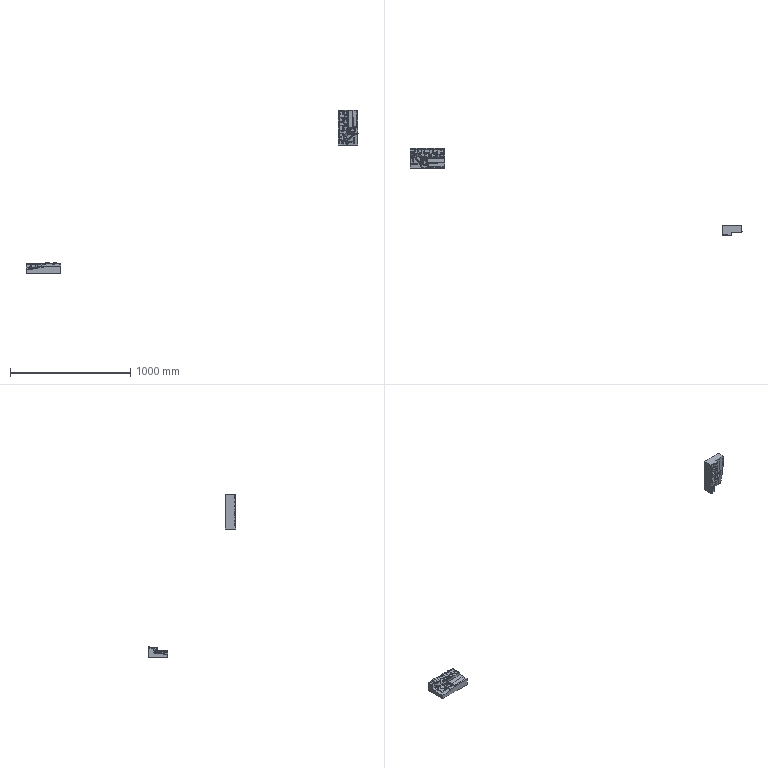NC program | NX | posted with a generic post | part box 2756 x 729.572 x 1353 mm
Lines 11439 to 12353 of 180527:
(CAVITY_MILL_COPY , TOOL : D12)
N22876 M6
N22878 G54
N22880 G17 G0 G90 X258.019 Y147.742 B0. C0. S3000 M3
N22882 G43 Z10. H0
N22884 Z-0.377
N22886 G94 G1 Z-0.577 F2500.
N22888 G3 X254.644 Y150.314 R3.5
N22890 G1 X232.072 Y150.313
N22892 G3 X228.608 Y147.313 R3.5
N22894 G1 Z-0.377
N22896 G0 Z0.3
N22898 X261.478 Y148.624
N22900 Z-0.954
N22902 G1 Z-1.154
N22904 G3 X257.802 Y150.414 R3.5
N22906 G2 X256.839 Y150.324 R6.307
N22908 G1 X256.382 Y150.316
N22910 X225.009 Y150.313
N22912 G2 X223.607 Y150.469 R6.345
N22914 G3 X219.842 Y148.871 R3.5
N22916 G1 Z-0.954
N22918 G0 Z-0.277
N22920 X264.623 Y150.548
N22922 Z-1.532
N22924 G1 Z-1.732
N22926 G3 X260.567 Y151.077 R3.5
N22928 G2 X257.569 Y150.32 R6.321
N22930 G1 X224.287 Y150.315
N22932 G2 X221.646 Y150.896 R6.285
N22934 G3 X217.502 Y149.979 R3.5
N22936 G1 Z-1.532
N22938 G0 Z10.
N22940 X243.577 Y116.823
N22942 Z-3.263
N22944 G1 Z-3.463
N22946 G3 X247.814 Y116.547 R3.5
N22948 G2 X253.823 Y118.323 R10.624
N22950 G1 X270.42 Y118.123
N22952 G3 X273.851 Y120.748 R3.5
N22954 G1 Z-3.263
N22956 G0 Z-2.586
N22958 X249.188 Y128.447
N22960 Z-3.84
N22962 G1 Z-4.04
N22964 G3 X252.126 Y127.231 R3.5
N22966 G2 X253.906 Y127.29 R19.545
N22968 G1 X260.583 Y127.271
N22970 G3 X263.387 Y128.664 R3.5
N22972 G1 Z-3.84
N22974 G0 Z-3.163
N22976 X241.75 Y116.424
N22978 Z-3.84
N22980 G1 Z-4.04
N22982 G3 X246.015 Y116.654 R3.5
N22984 G2 X253.808 Y119.491 R11.745
N22986 G1 X254.666 Y119.479
N22988 X270.111 Y119.448
N22990 X270.969 Y119.441
N22992 G2 X275.15 Y118.659 R11.535
N22994 G3 X279.245 Y119.86 R3.5
N22996 G1 Z-3.84
N22998 G0 Z10.
N23000 X287.438 Y92.406
N23002 Z-5.608
N23004 G1 Z-5.808
N23006 G3 X283.338 Y91.038 R3.5
N23008 G2 X275.259 Y85.078 R14.56
N23010 G1 X272.363 Y84.483
N23012 G3 X269.568 Y80.991 R3.5
N23014 G1 Z-5.608
N23016 G0 Z10.
N23018 X272.796 Y45.22
N23020 Z-28.229
N23022 G1 Z-28.429
N23024 G3 X276.749 Y46.24 R3.5
N23026 G2 X279.55 Y48.148 R6.196
N23028 X286.295 Y49.467 R22.571
N23030 X289.63 Y48.639 R6.145
N23032 G3 X293.691 Y49.029 R3.5
N23034 G1 Z-28.229
N23036 G0 Z10.
N23038 X274.725 Y81.825
N23040 Z-5.608
N23042 G1 Z-5.808
N23044 G3 X271.263 Y84.357 R3.5
N23046 X256.382 Y83.843 R1141.902
N23048 G2 X253.808 Y83.435 R10.93
N23050 X253.403 Y83.314 R11.557
N23052 G3 X250.847 Y79.897 R3.5
N23054 G1 Z-5.608
N23056 G0 Z10.
N23058 X293.281 Y79.065
N23060 Z-23.467
N23062 G1 Z-23.667
N23064 G3 X289.254 Y79.765 R3.5
N23066 G2 X286.414 Y79.134 R6.294
N23068 G1 X281.266
N23070 X257.82 Y79.033
N23072 G3 X254.369 Y76.018 R3.5
N23074 G1 Z-23.467
N23076 G0 Z-5.508
N23078 X294.249 Y80.286
N23080 Z-24.062
N23082 G1 Z-24.262
N23084 G3 X290.161 Y80.303 R3.5
N23086 G2 X286.414 Y79.134 R6.294
N23088 G1 X281.266
N23090 X234.553 Y78.933
N23092 G3 X231.102 Y75.918 R3.5
N23094 G1 Z-24.062
N23096 G0 Z-5.508
N23098 X295.018 Y81.695
N23100 Z-24.657
N23102 G1 Z-24.857
N23104 G3 X290.988 Y81.008 R3.5
N23106 G2 X286.414 Y79.134 R6.293
N23108 G1 X281.266
N23110 X211.763 Y78.835
N23112 X211.267 Y78.833
N23114 G3 X207.815 Y75.819 R3.5
N23116 G1 Z-24.657
N23118 G0 Z-5.508
N23120 X295.499 Y83.081
N23122 Z-25.252
N23124 G1 Z-25.452
N23126 G3 X291.627 Y81.768 R3.5
N23128 G2 X286.414 Y79.134 R6.293
N23130 G1 X281.266
N23132 X211.763 Y78.835
N23134 X188.052 Y78.737
N23136 G3 X184.6 Y75.723 R3.5
N23138 G1 Z-25.252
N23140 G0 Z-5.508
N23142 X295.647 Y83.746
N23144 Z-25.848
N23146 G1 Z-26.048
N23148 G3 X291.882 Y82.154 R3.5
N23150 G2 X286.414 Y79.134 R6.293
N23152 G1 X281.266
N23154 X211.763 Y78.835
N23156 X164.884 Y78.641
N23158 G3 X161.432 Y75.627 R3.5
N23160 G1 Z-25.848
N23162 G0 Z-5.508
N23164 X295.736 Y84.341
N23166 Z-26.443
N23168 G1 Z-26.643
N23170 G3 X292.082 Y82.508 R3.5
N23172 G2 X286.414 Y79.134 R6.294
N23174 G1 X281.266
N23176 X211.763 Y78.835
N23178 X142.852 Y78.55
N23180 G3 X139.4 Y75.531 R3.5
N23182 G1 Z-26.443
N23184 G0 Z-5.508
N23186 X295.79 Y84.974
N23188 Z-27.038
N23190 G1 Z-27.238
N23192 G3 X292.275 Y82.886 R3.5
N23194 G2 X286.414 Y79.106 R6.299
N23196 G1 X274.401 Y79.095
N23198 X212.621 Y78.842
N23200 X211.763 Y78.835
N23202 X141.402 Y78.543
N23204 X137.97 Y78.524
N23206 X132.679 Y78.512
N23208 G3 X129.221 Y75.504 R3.5
N23210 G1 Z-27.038
N23212 G0 Z-5.508
N23214 X295.8 Y85.303
N23216 Z-27.634
N23218 G1 Z-27.834
N23220 G3 X292.389 Y83.049 R3.5
N23222 G2 X286.414 Y78.993 R6.293
N23224 G3 X169.718 Y78.663 R25996.629
N23226 G1 X168.86 Y78.658
N23228 X129.389 Y78.501
N23230 X124.675 Y78.495
N23232 G3 X121.215 Y75.49 R3.5
N23234 G1 Z-27.634
N23236 G0 Z-26.938
N23238 X288.226 Y69.65
N23240 Z-28.229
N23242 G1 Z-28.429
N23244 G3 X285.492 Y70.97 R3.5
N23246 X275.305 Y70.983 R23551.141
N23248 X272.338 Y69.347 R3.5
N23250 G1 Z-28.229
N23252 G0 Z-5.508
N23254 X295.8 Y85.598
N23256 Z-28.229
N23258 G1 Z-28.429
N23260 G3 X292.5 Y83.164 R3.5
N23262 G2 X286.414 Y78.769 R6.319
N23264 G3 X134.537 Y78.511 R23558.941
N23266 G1 X122.947 Y78.492
N23268 G3 X119.488 Y75.491 R3.5
N23270 G1 Z-28.229
N23272 G0 Z-27.534
N23274 X255.498 Y58.426
N23276 Z-28.824
N23278 G1 Z-29.024
N23280 X261.061 Y58.625
N23282 G2 X257.876 Y62.414 R3.5
N23284 G3 X257.626 Y64.719 R6.
N23286 G2 X276.569 Y64.668 R26364.575
N23288 G1 X276.396 Y64.577
N23290 G3 X274.58 Y64.207 R43.297
N23292 G1 X260.992 Y62.763
N23294 X260.025 Y62.669
N23296 G3 X259.779 Y62.64 R6.
N23298 X257.895 Y62.349 R63.588
N23300 G2 X258.426 Y56.351 R16.06
N23302 X260.605 Y56.697 R57.588
N23304 G1 X261.599 Y56.793
N23306 X275.575 Y58.279
N23308 G2 X278.339 Y58.821 R37.297
N23310 G1 X280.04 Y59.713
N23312 G2 X286.156 Y61.301 R13.929
N23314 X287.712 Y70.688 R16.616
N23316 X286.359 Y70.636 R14.107
N23318 G3 X252.181 Y70.732 R26370.575
N23320 X249.227 Y69.12 R3.5
N23322 G1 Z-28.824
N23324 G0 Z-28.129
N23326 X248.852 Y38.697
N23328 Z-28.824
N23330 G1 Z-29.024
N23332 G3 X251.677 Y41.983 R3.5
N23334 G2 X256.439 Y48.002 R6.54
N23336 G1 X257.24 Y48.148
N23338 G2 X261.53 Y48.95 R49.788
N23340 G1 X262.388 Y49.033
N23342 X276.915 Y50.578
N23344 G2 X280.752 Y51.279 R29.497
N23346 G1 X283.662 Y52.805
N23348 G2 X290.517 Y52.012 R6.129
N23350 G3 X294.579 Y51.64 R3.5
N23352 G1 Z-28.824
N23354 G0 Z-28.129
N23356 X295.8 Y85.254
N23358 Z-28.824
N23360 G1 Z-29.024
N23362 G3 X292.5 Y82.821 R3.5
N23364 G2 X286.414 Y78.436 R6.307
N23366 G3 X121.955 Y78.49 R26378.375
N23368 X118.501 Y75.497 R3.5
N23370 G1 Z-28.824
N23372 G0 Z-28.129
N23374 X232.166 Y56.877
N23376 Z-29.419
N23378 G1 Z-29.619
N23380 G3 X235.099 Y56.036 R3.5
N23382 G2 X237.954 Y56.417 R37.22
N23384 G3 X254.609 Y58.255 R534.73
N23386 G1 X254.65 Y58.285
N23388 X255.308 Y58.867
N23390 X252.205 Y64.002
N23392 G2 X237.39 Y62.391 R528.73
N23394 G3 X235.102 Y62.113 R43.22
N23396 X234.861 Y64.429 R6.
N23398 G1 X252.789 Y64.327
N23400 X252.436 Y64.135
N23402 G3 X252.205 Y64.002 R6.
N23404 G1 X255.308 Y58.867
N23406 X256.08 Y59.288
N23408 G3 X264.143 Y64.097 R121.385
N23410 G1 X264.711 Y64.466
N23412 X265.334 Y64.732
N23414 G3 X272.592 Y68.306 R74.324
N23416 G1 X273.85 Y68.882
N23418 X276.947 Y70.19
N23420 X284.541 Y71.488
N23422 X276.947 Y70.19
N23424 X229.101 Y70.462
N23426 G3 X226.153 Y68.88 R3.5
N23428 G1 Z-29.419
N23430 G0 Z-28.724
N23432 X225.113 Y42.718
N23434 Z-29.419
N23436 G1 Z-29.619
N23438 G3 X228.81 Y44.451 R3.5
N23440 G2 X232.291 Y47.319 R6.202
N23442 X238.688 Y48.652 R29.42
N23444 G3 X256.07 Y50.578 R542.53
N23446 X259.814 Y52.439 R8.062
N23448 X268.395 Y57.558 R129.185
N23450 X276.117 Y61.342 R82.124
N23452 G1 X276.991 Y61.742
N23454 X283.84 Y64.634
N23456 X284.698 Y64.957
N23458 G2 X291.84 Y62.119 R6.215
N23460 G3 X295.566 Y60.448 R3.5
N23462 G1 Z-29.419
N23464 G0 Z-28.724
N23466 X295.8 Y84.806
N23468 Z-29.419
N23470 G1 Z-29.619
N23472 G3 X292.5 Y82.368 R3.5
N23474 G2 X286.414 Y77.937 R6.361
N23476 G1 X228.066 Y78.268
N23478 G3 X147.408 Y78.405 R29571.975
N23480 G2 X143.976 Y78.549 R45.359
N23482 G1 X121.142 Y78.49
N23484 G3 X117.689 Y75.505 R3.5
N23486 G1 Z-29.419
N23488 G0 Z-28.724
N23490 X208.927 Y56.778
N23492 Z-30.015
N23494 G1 Z-30.215
N23496 G3 X211.833 Y55.71 R3.5
N23498 G1 X212.555 Y55.787
N23500 X211.921 Y61.754
N23502 G3 X211.685 Y64.1 R6.
N23504 G2 X229.024 Y63.967 R11013.816
N23506 G1 X228.464 Y63.56
N23508 X227.582 Y63.395
N23510 X224.975 Y63.14
N23512 X224.925 Y63.135
N23514 X211.921 Y61.754
N23516 X212.555 Y55.787
N23518 X225.559 Y57.169
N23520 X228.427 Y57.449
N23522 X230.899 Y57.911
N23524 X233.908 Y60.101
N23526 X236.021 Y61.971
N23528 X236.785 Y62.461
N23530 X242.064 Y65.713
N23532 X243.368 Y66.601
N23534 X248.69 Y69.783
N23536 X255.094 Y71.253
N23538 X248.69 Y69.783
N23540 G3 X206.139 Y70.137 R11019.816
N23542 X203.21 Y68.587 R3.5
N23544 G1 Z-30.015
N23546 G0 Z-29.319
N23548 X202.061 Y44.372
N23550 Z-30.015
N23552 G1 Z-30.215
N23554 G3 X206.055 Y45.196 R3.5
N23556 G2 X208.589 Y46.841 R6.116
N23558 G1 X209.48 Y47.143
N23560 X212.621 Y47.878
N23562 X213.106 Y48.002
N23564 X226.35 Y49.409
N23566 X229.524 Y49.719
N23568 X234.119 Y50.578
N23570 X234.93 Y51.199
N23572 X238.799 Y54.013
N23574 X240.739 Y55.73
N23576 X240.937 Y55.857
N23578 X246.306 Y59.165
N23580 X247.568 Y60.024
N23582 X253.312 Y63.459
N23584 G3 X266.679 Y69.997 R551.817
N23586 X283.84 Y76.474 R770.832
N23588 G1 X284.698 Y76.79
N23590 G2 X292.5 Y72.288 R6.182
N23592 G1 Y72.453
N23594 G2 X292.445 Y74.338 R18.838
N23596 G3 X292.44 Y74.738 R6.15
N23598 G2 X292.428 Y76.152 R19.559
N23600 G3 X292.428 Y76.484 R6.15
N23602 G2 X292.463 Y78.295 R20.078
N23604 G3 X292.475 Y78.746 R6.15
N23606 G2 X292.5 Y79.968 R20.632
N23608 G1 Y81.636
N23610 G2 X286.414 Y77.185 R6.386
N23612 G1 X282.982 Y77.183
N23614 X274.588 Y77.288
N23616 G3 X147.675 Y78.156 R11027.616
N23618 G2 X143.497 Y78.487 R26.864
N23620 G3 X142.276 Y78.54 R13.208
N23622 G1 X121.666 Y78.485
N23624 X118.853 Y78.486
N23626 G3 X115.402 Y75.575 R3.5
N23628 G1 Z-30.015
N23630 G0 Z-29.319
N23632 X185.746 Y56.228
N23634 Z-30.61
N23636 G1 Z-30.81
N23638 G3 X188.654 Y55.331 R3.5
N23640 G2 X189.288 Y55.421 R33.99
N23642 G1 X188.499 Y61.369
N23644 G3 X188.27 Y63.727 R6.
N23646 G2 X204.462 Y63.553 R7262.398
N23648 X203.967 Y63.083 R99.069
N23650 X190.027 Y61.542 R419.884
N23652 G3 X188.499 Y61.369 R39.99
N23654 G1 X189.288 Y55.421
N23656 G2 X190.586 Y55.568 R33.99
N23658 G3 X206.637 Y57.379 R425.884
N23660 X211.77 Y62.37 R105.069
N23662 G2 X215.077 Y65.233 R23.829
N23664 G1 X216.933 Y66.989
N23666 G2 X219.98 Y69.353 R19.806
N23668 G1 X225.808 Y71.03
N23670 X219.98 Y69.353
N23672 G3 X183.313 Y69.774 R7268.398
N23674 X180.399 Y68.259 R3.5
N23676 G1 Z-30.61
N23678 G0 Z-29.915
N23680 X178.262 Y43.049
N23682 Z-30.61
N23684 G1 Z-30.81
N23686 G3 X182.149 Y44.291 R3.5
N23688 G2 X185.044 Y46.425 R6.161
N23690 X191.313 Y47.802 R26.19
N23692 G3 X208.205 Y49.719 R433.684
N23694 G1 X208.331 Y49.748
N23696 X210.047 Y50.109
N23698 G2 X210.305 Y50.201 R0.139
N23700 G3 X217.395 Y56.966 R112.869
N23702 G2 X220.013 Y59.165 R16.029
N23704 G1 X222.293 Y61.322
N23706 G2 X225.424 Y63.459 R12.006
N23708 G1 X231.727 Y67.753
N23710 X240.079 Y73.035
N23712 X240.937 Y73.495
N23714 X248.363 Y76.702
N23716 G3 X146.55 Y77.809 R7276.198
N23718 G2 X142.799 Y78.418 R24.764
N23720 G3 X141.725 Y78.544 R4.504
N23722 G1 X124.241 Y78.49
N23724 X123.383 Y78.467
N23726 G2 X116.518 Y78.495 R100.431
N23728 G1 X115.66 Y78.515
N23730 G2 X114.853 Y78.559 R58.457
N23732 G3 X111.225 Y75.845 R3.5
N23734 G1 Z-30.61
N23736 G0 Z10.
N23738 X117.471 Y75.263
N23740 Z-30.61
N23742 G1 Z-30.81
N23744 G3 X114.227 Y78.601 R3.5
N23746 G2 X98.316 Y82.028 R58.457
N23748 G3 X94.08 Y80.495 R3.5
N23750 G1 Z-30.61
N23752 G0 Z-29.915
N23754 X162.714 Y60.178
N23756 Z-31.205
N23758 G1 Z-31.405
N23760 X167.207 Y61.092
N23762 G2 X165.193 Y62.53 R1.75
N23764 G3 X165.019 Y63.274 R6.
N23766 G2 X179.096 Y63.071 R4049.216
N23768 G1 X178.639 Y62.374
N23770 X177.783 Y62.291
N23772 X177.723 Y62.285
N23774 X165.61 Y60.985
N23776 G2 X165.763 Y54.967 R16.06
N23778 G1 X165.885 Y54.98
N23780 X178.363 Y56.319
N23782 X181.153 Y56.591
N23784 X182.139 Y56.775
N23786 X184.251 Y59.99
N23788 X184.446 Y60.291
N23790 G2 X187.397 Y64.687 R16.809
N23792 G3 X191.074 Y68.861 R101.161
N23794 X160.864 Y69.325 R4055.216
N23796 X157.972 Y67.854 R3.5
N23798 G1 Z-31.205
N23800 G0 Z-30.51
N23802 X155.534 Y44.019
N23804 Z-31.205
N23806 G1 Z-31.405
N23808 G3 X159.566 Y44.63 R3.5
N23810 G2 X161.802 Y46.017 R6.114
N23812 G1 X162.561 Y46.284
N23814 X165.428 Y46.999
N23816 X165.956 Y47.143
N23818 X179.157 Y48.56
N23820 X182.25 Y48.86
N23822 X186.836 Y49.719
N23824 X190.785 Y55.73
N23826 X191.341 Y56.589
N23828 G2 X193.107 Y59.373 R9.009
N23830 G3 X198.394 Y65.494 R108.961
N23832 G2 X199.867 Y66.921 R8.171
N23834 G3 X204.613 Y71.188 R36.191
N23836 G2 X206.788 Y73.512 R6.9
N23838 G1 X210.896 Y76.237
N23840 G3 X147.124 Y77.261 R4063.016
N23842 G2 X143.071 Y78.058 R11.175
N23844 G1 X141.667 Y78.487
N23846 X141.402 Y78.529
N23848 X140.544 Y78.536
N23850 X126.815 Y78.495
N23852 X125.957 Y78.478
N23854 X125.099 Y78.445
N23856 G2 X115.66 Y78.441 R116.512
N23858 X98.529 Y81.775 R59.292
N23860 G3 X94.313 Y80.194 R3.5
N23862 G1 Z-31.205
N23864 G0 Z-30.51
N23866 X145.408 Y61.356
N23868 Z-31.801
N23870 G1 Z-32.001
N23872 G2 X148.169 Y62.584 R3.5
N23874 G1 X151.606 Y62.489
N23876 G2 X151.379 Y61.442 R254.449
N23878 G1 X148.563 Y61.131
N23880 G2 X148.791 Y55.12 R16.616
N23882 G1 X156.282 Y55.946
N23884 G3 X157.791 Y62.738 R260.449
N23886 G1 X157.926 Y63.386
N23888 X158.606 Y65.118
N23890 X160.392 Y68.248
N23892 X145.933 Y68.649
N23894 X145.534 Y68.701
N23896 G2 X144.636 Y68.84 R19.355
N23898 G3 X141.498 Y67.825 R3.5
N23900 G1 Z-31.801
N23902 G0 Z-31.105
N23904 X140.016 Y45.423
N23906 Z-31.801
N23908 G1 Z-32.001
N23910 G3 X144.147 Y45.613 R3.5
N23912 G2 X147.798 Y47.163 R7.263
N23914 G1 X159.421 Y48.445
N23916 X161.995 Y48.956
N23918 X162.283 Y49.04
N23920 X162.446 Y49.206
N23922 X162.621 Y49.073
N23924 G3 X165.428 Y61.149 R268.249
N23926 G1 X165.66 Y61.742
N23928 X168.6 Y66.894
N23930 X169.473 Y69.47
N23932 X171.529 Y72.905
N23934 G2 X172.895 Y75.698 R6.993
N23936 G1 X172.432 Y75.717
N23938 X146.55 Y76.434
N23940 G2 X142.26 Y77.894 R11.555
N23942 G3 X141.058 Y78.432 R4.899
N23944 X129.389 Y78.5 R423.334
N23946 X122.524 Y78.228 R342.74
N23948 G2 X110.512 Y78.749 R81.577
N23950 X104.107 Y79.929 R57.626
N23952 G3 X100.069 Y77.926 R3.5
N23954 G1 Z-31.801
N23956 G0 Z-31.105
N23958 X137.24 Y39.552
N23960 Z-32.396
N23962 G1 Z-32.596
N23964 G3 X140.527 Y42.185 R3.5
N23966 X140.96 Y44.567 R17.278
N23968 G1 X140.942 Y45.457
N23970 G3 X137.872 Y48.859 R3.5
N23972 G1 Z-32.396
N23974 G0 Z10.
N23976 X138.44 Y-6.669
N23978 Z-34.182
N23980 G1 Z-34.382
N23982 G3 X139.182 Y-2.643 R3.5
N23984 G2 X138.568 Y-0.088 R6.396
N23986 G1 X138.525 Y0.771
N23988 X137.923 Y39.734
N23990 G3 X134.87 Y43.151 R3.5
N23992 G1 Z-34.182
N23994 G0 Z10.
N23996 X125.958 Y27.196
N23998 Z-35.372
N24000 G1 Z-35.572
N24002 G3 X130.141 Y28.404 R3.5
N24004 X132.606 Y33.403 R17.462
N24006 X133.047 Y37.068 R13.578
N24008 G1 X133.027 Y38.266
N24010 G3 X129.97 Y41.68 R3.5
N24012 G1 Z-35.372
N24014 G0 Z-34.082
N24016 X119.184 Y25.255
N24018 Z-35.968
N24020 G1 Z-36.168
N24022 G3 X123.349 Y25.264 R3.5
N24024 G2 X123.957 Y25.674 R8.
N24026 G1 X124.241 Y25.815
N24028 G3 X127.506 Y27.922 R83.682
N24030 X132.234 Y37.041 R10.785
N24032 G1 X132.191 Y39.414
N24034 X132.08 Y45.827
N24036 G3 X129.02 Y49.239 R3.5
N24038 G1 Z-35.968
N24040 G0 Z10.
N24042 X133.018 Y68.46
N24044 Z-32.396
N24046 G1 Z-32.596
N24048 G3 X134.411 Y71.327 R3.5
N24050 G1 X134.389 Y72.392
N24052 G3 X133.239 Y72.403 R306.312
N24054 X130.341 Y70.905 R3.5
N24056 G1 Z-32.396
N24058 G0 Z-31.701
N24060 X137.731 Y55.732
N24062 Z-32.396
N24064 G1 Z-32.596
N24066 G3 X140.659 Y59.257 R3.5
N24068 G1 X140.27 Y78.271
N24070 G3 X130.247 Y78.412 R312.312
N24072 X123.383 Y78.061 R253.148
N24074 G2 X117.609 Y78.031 R51.104
N24076 G3 X113.996 Y75.213 R3.5
N24078 G1 Z-32.396
N24080 G0 Z-31.701
N24082 X131.716 Y68.965
N24084 Z-32.991
N24086 G1 Z-33.191
N24088 G3 X133.096 Y71.813 R3.5
N24090 G1 X133.089 Y72.205
N24092 X132.668 Y72.218
N24094 X132.644 Y72.219
N24096 G3 X129.708 Y70.737 R3.5
N24098 G1 Z-32.991
N24100 G0 Z-32.296
N24102 X136.38 Y55.982
N24104 Z-32.991
N24106 G1 Z-33.191
N24108 G3 X139.317 Y59.5 R3.5
N24110 G1 X138.985 Y78.021
N24112 X132.821 Y78.216
N24114 X132.658 Y78.22
N24116 G3 X126.063 Y77.958 R55.731
N24118 G2 X119.092 Y77.703 R54.879
N24120 G1 X117.376 Y77.765
N24122 G2 X114.685 Y77.905 R82.586
N24124 G3 X111.04 Y75.217 R3.5
N24126 G1 Z-32.991
N24128 G0 Z-32.296
N24130 X130.975 Y68.678
N24132 Z-33.586
N24134 G1 Z-33.786
N24136 G3 X132.342 Y71.513 R3.5
N24138 G1 X132.335 Y71.899
N24140 X131.871 Y71.92
N24142 G3 X128.859 Y70.452 R3.5
N24144 G1 Z-33.586
N24146 G0 Z-32.891
N24148 X135.616 Y55.5
N24150 Z-33.586
N24152 G1 Z-33.786
N24154 G3 X138.557 Y59.015 R3.5
N24156 G1 X138.238 Y77.636
N24158 X131.963 Y77.922
N24160 X131.105 Y77.936
N24162 G3 X125.099 Y77.534 R81.897
N24164 G2 X119.092 Y77.35 R40.053
N24166 G1 X117.376 Y77.429
N24168 G2 X115.994 Y77.494 R85.299
N24170 G3 X112.385 Y74.756 R3.5
N24172 G1 Z-33.586
N24174 G0 Z-32.891
N24176 X130.071 Y68.48
N24178 Z-34.182
N24180 G1 Z-34.382
N24182 G3 X131.435 Y71.307 R3.5
N24184 G1 X131.432 Y71.496
N24186 X131.208 Y71.503
N24188 G3 X128.237 Y70.021 R3.5
N24190 G1 Z-34.182
N24192 G0 Z-33.486
N24194 X134.679 Y55.49
N24196 Z-34.182
N24198 G1 Z-34.382
N24200 G3 X137.626 Y59. R3.5
N24202 G1 X137.346 Y77.107
N24204 X131.963 Y77.482
N24206 X131.105 Y77.509
N24208 G3 X125.099 Y77.067 R68.258
N24210 G2 X119.092 Y76.904 R36.641
N24212 G1 X117.376 Y77.002
N24214 X114.65 Y77.177
N24216 G2 X112.653 Y77.333 R70.405
N24218 G3 X108.947 Y74.746 R3.5
N24220 G1 Z-34.182
N24222 G0 Z-33.486
N24224 X128.336 Y67.488
N24226 Z-34.777
N24228 G1 Z-34.977
N24230 G3 X129.697 Y70.28 R3.5
N24232 G1 X129.694 Y70.841
N24234 G3 X129.021 Y70.811 R23.621
N24236 X126.211 Y69.092 R3.5
N24238 G1 Z-34.777
N24240 G0 Z-34.082
N24242 X132.81 Y51.957
N24244 Z-34.777
N24246 G1 Z-34.977
N24248 G3 X135.788 Y55.44 R3.5
N24250 G1 X135.66 Y76.384
N24252 G3 X126.518 Y76.594 R29.621
N24254 G2 X117.376 Y76.461 R39.055
N24256 X112.146 Y76.894 R102.255
N24258 G3 X108.392 Y74.342 R3.5
N24260 G1 Z-34.777
N24262 G0 Z-34.082
N24264 X129.768 Y53.859
N24266 Z-35.372
N24268 G1 Z-35.572
N24270 G3 X132.71 Y57.372 R3.5
N24272 G1 X132.707 Y57.54
N24274 G3 X130.119 Y65.557 R14.454
N24276 G2 X128.19 Y70.329 R11.594
N24278 G1 X128.194 Y75.825
N24280 G2 X115.66 Y75.931 R48.69
N24282 X106.234 Y77.169 R73.542
N24284 G1 X106.233 Y77.166
N24286 X106.236
N24288 Z-35.372
N24290 G0 Z-34.677
N24292 X129.069 Y46.421
N24294 Z-35.968
N24296 G1 Z-36.168
N24298 G3 X132.008 Y49.936 R3.5
N24300 G1 X131.878 Y57.448
N24302 G3 X128.531 Y65.233 R10.663
N24304 X125.957 Y67.311 R26.107
N24306 G2 X124.241 Y68.416 R9.424
N24308 X123.465 Y68.918 R7.552
N24310 G3 X119.046 Y68.702 R3.5
N24312 G1 Z-35.968
N24314 G0 Z-35.272
N24316 X113.409 Y26.779
N24318 Z-36.563
N24320 G1 Z-36.763
N24322 G3 X117.385 Y25.688 R3.5
N24324 G1 X117.554 Y25.749
N24326 G2 X123.159 Y27.205 R35.268
N24328 G3 X129.584 Y30.827 R11.015
N24330 X131.722 Y36.838 R9.155
N24332 G1 X131.357 Y57.448
N24334 G3 X127.423 Y65.141 R9.425
N24336 X122.339 Y67.232 R11.971
N24338 G2 X117.895 Y68.366 R25.168
N24340 G3 X113.905 Y67.142 R3.5
N24342 G1 Z-36.563
N24344 G0 Z-35.868
N24346 X109.56 Y30.711
N24348 Z-37.158
N24350 G1 Z-37.358
N24352 G3 X112.832 Y28.211 R3.5
N24354 G2 X113.944 Y28.094 R6.887
N24356 G3 X119.092 Y27.617 R27.823
N24358 G1 X119.95 Y27.688
N24360 X123.383 Y28.097
N24362 G3 X129.724 Y31.686 R9.168
N24364 X131.372 Y36.838 R8.406
N24366 G1 X130.993 Y57.448
N24368 X130.959 Y58.307
N24370 G3 X126.314 Y65.177 R8.579
N24372 X121.666 Y66.336 R10.75
N24374 X113.944 Y66.312 R27.601
N24376 G2 X113.412 Y66.249 R6.953
N24378 G3 X110.279 Y63.572 R3.5
N24380 G1 Z-37.158
N24382 G0 Z-36.463
N24384 X105.417 Y45.131
N24386 Z-37.753
N24388 G1 Z-37.953
N24390 G3 X108.005 Y43.082 R3.5
N24392 G2 X112.852 Y41.242 R14.164
N24394 G1 X113.338 Y40.946
N24396 X115.999 Y47.53
N24398 X113.338 Y40.946
N24400 X114.733 Y39.957
N24402 X115.748 Y38.848
N24404 G3 X117.924 Y36.829 R81.069
N24406 X119.852 Y36.184 R2.57
N24408 G1 X122.995 Y36.446
N24410 G3 X123.25 Y36.573 R0.387
N24412 G1 X123.302 Y36.646
N24414 X123.281 Y36.734
N24416 G2 X122.909 Y57.422 R3980.562
N24418 G1 X122.91 Y57.516
N24420 G3 X122.772 Y57.798 R0.352
N24422 X122.233 Y57.877 R1.685
N24424 G1 X119.388 Y58.013
N24426 G3 X117.221 Y57.241 R3.027
N24428 G2 X114.024 Y54.627 R44.656
N24430 X108.025 Y52.04 R14.189
N24432 G3 X105.429 Y50. R3.5
N24434 G1 Z-37.753
N24436 G0 Z-37.058
N24438 X96.077 Y28.904
N24440 Z-37.753
N24442 G1 Z-37.953
N24444 G3 X99.48 Y31.247 R3.5
N24446 G2 X108.796 Y34.579 R6.364
N24448 G1 X109.178 Y34.262
N24450 X109.654 Y33.954
N24452 X110.158 Y33.403
N24454 G3 X112.725 Y31.015 R88.869
N24456 X120.501 Y28.411 R10.37
N24458 G1 X123.645 Y28.674
N24460 G3 X129.937 Y32.544 R8.187
N24462 X131.081 Y36.838 R8.273
N24464 G2 X130.709 Y57.448 R3972.762
N24466 G3 X125.957 Y64.928 R8.152
N24468 X122.524 Y65.672 R9.485
N24470 G1 X119.759 Y65.804
N24472 G3 X112.008 Y63.044 R10.827
N24474 G2 X109.37 Y60.886 R36.856
N24476 X99.762 Y63.324 R6.389
N24478 G3 X96.194 Y65.329 R3.5
N24480 G1 Z-37.753
N24482 G0 Z-37.058
N24484 X122.731 Y46.921
N24486 Z-37.753
N24488 G3 X122.731 Y46.921 Z-38.543 I-4.798 J0.124
N24490 X122.732 Y47.132 Z-38.549 R4.8
N24492 G1 X122.55 Y57.184
N24494 X122.536 Y57.463
N24496 X119.689 Y57.564
N24498 G3 X119.052 Y57.311 R0.868
N24500 G1 X119.516 Y36.882
N24502 G3 X119.642 Y36.722 R0.169
N24504 G1 X119.909 Y36.652
N24506 G3 X120.185 Y36.628 R0.834
N24508 G1 X120.253 Y36.633
N24510 X122.919 Y36.8
N24512 X122.732 Y47.132
N24514 X130.531 Y47.273
N24516 X130.347 Y57.448
N24518 X130.315 Y58.087
N24520 G3 X124.54 Y65.039 R7.529
N24522 X122.952 Y65.254 R8.085
N24524 G1 X119.95 Y65.36
N24526 G3 X112.616 Y61.742 R8.668
N24528 X111.247 Y57.448 R7.31
N24530 G1 X111.718 Y36.705
N24532 G3 X117.649 Y29.181 R7.969
N24534 G1 X117.921 Y29.109
N24536 G3 X120.808 Y28.853 R8.634
N24538 G1 X123.383 Y29.014
N24540 G3 X130.72 Y36.838 R7.625
N24542 G1 X130.531 Y47.273
N24544 G3 X126.968 Y50.709 R3.5
N24546 G1 Z-38.349
N24548 G0 Z-37.653
N24550 X120.162 Y47.308
N24552 Z-38.349
N24554 G3 X120.162 Y47.308 Z-39.138 I4.799 J-0.111
N24556 X120.162 Y47.097 Z-39.144 R4.8
N24558 G1 X120.371 Y37.099
N24560 X120.375 Y37.008
N24562 G3 X122.421 Y37.138 R44.721
N24564 G1 X122.394 Y38.407
N24566 X122.076 Y57.124
N24568 X119.95 Y57.186
N24570 X119.959 Y56.752
N24572 X120.162 Y47.097
N24574 X112.363 Y46.934
N24576 X112.575 Y36.838
N24578 X112.614 Y35.979
N24580 G3 X119.95 Y29.19 R7.559
N24582 X124.241 Y29.479 R52.521
N24584 X130.229 Y36.838 R7.234
N24586 G1 X130.193 Y38.556
N24588 X129.866 Y57.81
N24590 G3 X122.858 Y64.904 R7.22
N24592 G1 X119.95 Y64.99
N24594 G3 X112.188 Y58.307 R7.602
N24596 G1 X112.143 Y57.448
N24598 X112.161 Y56.589
N24600 X112.363 Y46.934
N24602 G3 X112.902 Y45.707 R1.75
N24604 G1 Z-38.944
N24606 G0 Z-38.249
N24608 X121.789 Y50.055
N24610 Z-38.944
N24612 G3 X121.789 Y50.055 Z-39.655 I3.228 J-2.87
N24614 X120.699 Y47.097 Z-39.739 R4.32
N24616 G1 X120.895 Y37.439
N24618 G3 X121.715 Y37.504 R22.799
N24620 G1 X121.689 Y39.29
N24622 X121.393 Y56.748
N24624 G3 X120.87 Y56.758 R9.762
N24626 G1 X120.503 Y56.755
N24628 X120.699 Y47.097
N24630 X112.9 Y46.939
N24632 X113.105 Y36.838
N24634 X113.129 Y36.269
N24636 G3 X120.354 Y29.607 R6.956
N24638 G1 X120.808 Y29.625
N24640 G3 X123.76 Y29.893 R30.599
N24642 X129.529 Y36.627 R6.699
N24644 G1 X129.488 Y39.414
N24646 X129.182 Y57.448
N24648 X129.144 Y58.307
N24650 G3 X124.241 Y64.246 R6.757
N24652 X120.808 Y64.557 R17.562
N24654 X117.698 Y64.318 R9.066
N24656 X112.687 Y57.448 R7.084
N24658 G1 X112.9 Y46.939
N24660 G3 X116.471 Y43.51 R3.5
N24662 G1 Z-39.539
N24664 G0 Z-38.844
N24666 X121.641 Y44.78
N24668 Z-39.539
N24670 G3 X121.641 Y44.78 Z-40.27 I-3.805 J2.289
N24672 X122.276 Y47.137 Z-40.335 R4.44
N24674 G1 X122.119 Y57.217
N24676 X122.078 Y57.897
N24678 X119.582 Y58.061
N24680 G3 X119.109 Y57.582 R0.454
N24682 G1 X119.504 Y37.879
N24684 X119.563 Y36.443
N24686 G3 X119.784 Y36.163 R0.413
N24688 X121.554 Y36.3 R10.449
N24690 G1 X121.989 Y36.371
N24692 X122.393 Y36.378
N24694 X122.433 Y36.991
N24696 X122.276 Y47.137
N24698 X128.275 Y47.23